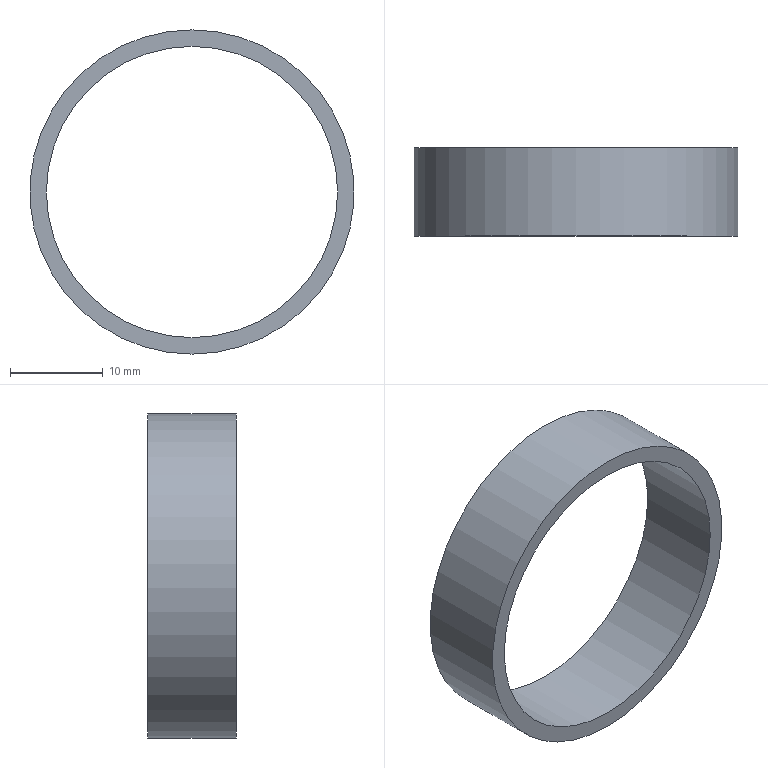Part | NX | features piston ring 2 | 1 solid | 4 faces | box 34.925 x 9.525 x 34.925 mm | volume 1764 mm3 | cylinder 2 | plane 2 | commonest cylinder face diameters 31.369 x1 34.925 x1
STEP:
#1=CARTESIAN_POINT('',(0.,-4.763,-15.684));
#2=VERTEX_POINT('',#1);
#3=CARTESIAN_POINT('',(0.,-4.763,0.));
#4=DIRECTION('',(0.,-1.,0.));
#5=DIRECTION('',(0.,0.,-1.));
#6=AXIS2_PLACEMENT_3D('',#3,#4,#5);
#7=CIRCLE('',#6,15.684);
#8=EDGE_CURVE('',#2,#2,#7,.T.);
#9=ORIENTED_EDGE('',*,*,#8,.T.);
#10=EDGE_LOOP('',(#9));
#11=FACE_BOUND('',#10,.T.);
#12=CARTESIAN_POINT('',(0.,4.763,-15.684));
#13=VERTEX_POINT('',#12);
#14=CARTESIAN_POINT('',(0.,4.763,0.));
#15=DIRECTION('',(0.,-1.,0.));
#16=DIRECTION('',(0.,0.,-1.));
#17=AXIS2_PLACEMENT_3D('',#14,#15,#16);
#18=CIRCLE('',#17,15.684);
#19=EDGE_CURVE('',#13,#13,#18,.T.);
#20=ORIENTED_EDGE('',*,*,#19,.F.);
#21=EDGE_LOOP('',(#20));
#22=FACE_BOUND('',#21,.T.);
#23=CARTESIAN_POINT('',(0.,0.,0.));
#24=DIRECTION('',(0.,-1.,0.));
#25=DIRECTION('',(0.,0.,-1.));
#26=AXIS2_PLACEMENT_3D('',#23,#24,#25);
#27=CYLINDRICAL_SURFACE('',#26,15.684);
#28=ADVANCED_FACE('',(#11,#22),#27,.F.);
#29=CARTESIAN_POINT('',(0.,-4.763,-17.462));
#30=VERTEX_POINT('',#29);
#31=CARTESIAN_POINT('',(0.,-4.763,0.));
#32=DIRECTION('',(0.,-1.,0.));
#33=DIRECTION('',(0.,0.,-1.));
#34=AXIS2_PLACEMENT_3D('',#31,#32,#33);
#35=CIRCLE('',#34,17.462);
#36=EDGE_CURVE('',#30,#30,#35,.T.);
#37=ORIENTED_EDGE('',*,*,#36,.T.);
#38=EDGE_LOOP('',(#37));
#39=FACE_BOUND('',#38,.T.);
#40=ORIENTED_EDGE('',*,*,#8,.F.);
#41=EDGE_LOOP('',(#40));
#42=FACE_BOUND('',#41,.T.);
#43=CARTESIAN_POINT('',(15.684,-4.763,0.));
#44=DIRECTION('',(0.,-1.,0.));
#45=DIRECTION('',(0.,0.,-1.));
#46=AXIS2_PLACEMENT_3D('',#43,#44,#45);
#47=PLANE('',#46);
#48=ADVANCED_FACE('',(#39,#42),#47,.T.);
#49=CARTESIAN_POINT('',(0.,4.763,-17.462));
#50=VERTEX_POINT('',#49);
#51=CARTESIAN_POINT('',(0.,4.763,0.));
#52=DIRECTION('',(0.,-1.,0.));
#53=DIRECTION('',(0.,0.,-1.));
#54=AXIS2_PLACEMENT_3D('',#51,#52,#53);
#55=CIRCLE('',#54,17.462);
#56=EDGE_CURVE('',#50,#50,#55,.T.);
#57=ORIENTED_EDGE('',*,*,#56,.T.);
#58=EDGE_LOOP('',(#57));
#59=FACE_BOUND('',#58,.T.);
#60=ORIENTED_EDGE('',*,*,#36,.F.);
#61=EDGE_LOOP('',(#60));
#62=FACE_BOUND('',#61,.T.);
#63=CARTESIAN_POINT('',(0.,0.,0.));
#64=DIRECTION('',(0.,-1.,0.));
#65=DIRECTION('',(0.,0.,-1.));
#66=AXIS2_PLACEMENT_3D('',#63,#64,#65);
#67=CYLINDRICAL_SURFACE('',#66,17.462);
#68=ADVANCED_FACE('',(#59,#62),#67,.T.);
#69=ORIENTED_EDGE('',*,*,#19,.T.);
#70=EDGE_LOOP('',(#69));
#71=FACE_BOUND('',#70,.T.);
#72=ORIENTED_EDGE('',*,*,#56,.F.);
#73=EDGE_LOOP('',(#72));
#74=FACE_BOUND('',#73,.T.);
#75=CARTESIAN_POINT('',(15.684,4.763,0.));
#76=DIRECTION('',(0.,1.,0.));
#77=DIRECTION('',(0.,0.,1.));
#78=AXIS2_PLACEMENT_3D('',#75,#76,#77);
#79=PLANE('',#78);
#80=ADVANCED_FACE('',(#71,#74),#79,.T.);
#81=CLOSED_SHELL('',(#28,#48,#68,#80));
#82=MANIFOLD_SOLID_BREP('',#81);
#83=(LENGTH_UNIT()NAMED_UNIT(*)SI_UNIT(.MILLI.,.METRE.));
#84=UNCERTAINTY_MEASURE_WITH_UNIT(LENGTH_MEASURE(0.00001),#83,'','');
#85=(NAMED_UNIT(*)PLANE_ANGLE_UNIT()SI_UNIT($,.RADIAN.));
#86=(NAMED_UNIT(*)SI_UNIT($,.STERADIAN.)SOLID_ANGLE_UNIT());
#87=(GEOMETRIC_REPRESENTATION_CONTEXT(3)GLOBAL_UNCERTAINTY_ASSIGNED_CONTEXT((#84))GLOBAL_UNIT_ASSIGNED_CONTEXT((#83,#85,#86))REPRESENTATION_CONTEXT('',''));
#88=ADVANCED_BREP_SHAPE_REPRESENTATION('',(#82),#87);